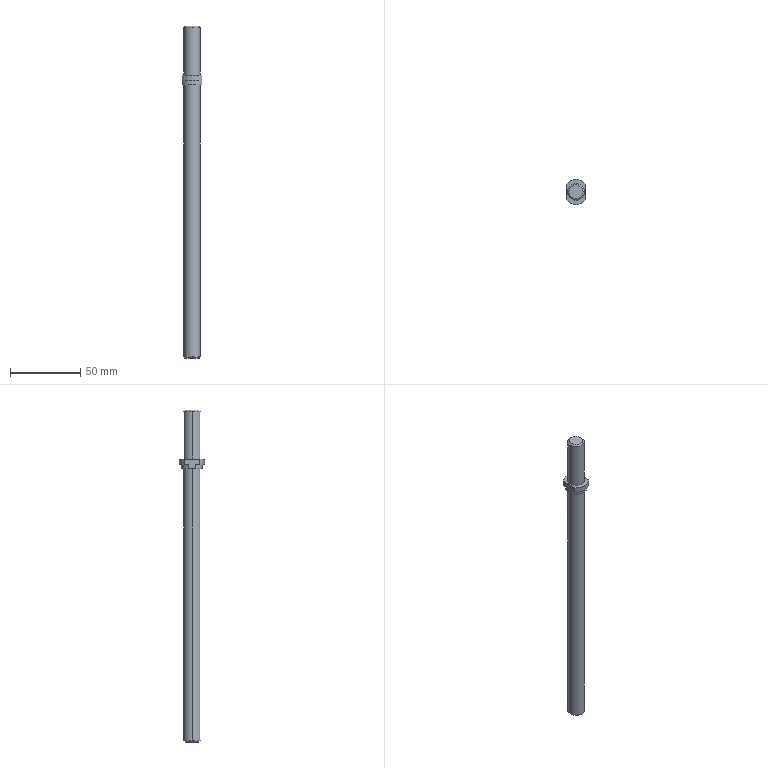Part | STEP file | MT-COMBO-119-S043 | 1 solid | 24 faces | box 14 x 18 x 237 mm | volume 27010 mm3 | cylinder 10 | plane 8 | cone 6 | commonest cylinder face diameters 12 x4 4.2 x2 15 x2 18 x2
STEP:
#1=CARTESIAN_POINT('',(2.1,0.,15.));
#2=VERTEX_POINT('',#1);
#3=CARTESIAN_POINT('',(-2.1,0.,15.));
#4=VERTEX_POINT('',#3);
#5=CARTESIAN_POINT('',(0.,0.,15.));
#6=DIRECTION('',(0.,0.,1.));
#7=DIRECTION('',(1.,0.,0.));
#8=AXIS2_PLACEMENT_3D('',#5,#6,#7);
#9=CIRCLE('',#8,2.1);
#10=EDGE_CURVE('',#2,#4,#9,.T.);
#11=ORIENTED_EDGE('',*,*,#10,.T.);
#12=CARTESIAN_POINT('',(-2.1,0.,-12.));
#13=VERTEX_POINT('',#12);
#14=CARTESIAN_POINT('',(-2.1,0.,0.));
#15=DIRECTION('',(0.,0.,-1.));
#16=VECTOR('',#15,1000.);
#17=LINE('',#14,#16);
#18=EDGE_CURVE('',#4,#13,#17,.T.);
#19=ORIENTED_EDGE('',*,*,#18,.T.);
#20=CARTESIAN_POINT('',(2.1,0.,-12.));
#21=VERTEX_POINT('',#20);
#22=CARTESIAN_POINT('',(0.,0.,-12.));
#23=DIRECTION('',(0.,0.,1.));
#24=DIRECTION('',(1.,0.,0.));
#25=AXIS2_PLACEMENT_3D('',#22,#23,#24);
#26=CIRCLE('',#25,2.1);
#27=EDGE_CURVE('',#21,#13,#26,.T.);
#28=ORIENTED_EDGE('',*,*,#27,.F.);
#29=CARTESIAN_POINT('',(2.1,0.,0.));
#30=DIRECTION('',(0.,0.,-1.));
#31=VECTOR('',#30,1000.);
#32=LINE('',#29,#31);
#33=EDGE_CURVE('',#2,#21,#32,.T.);
#34=ORIENTED_EDGE('',*,*,#33,.F.);
#35=EDGE_LOOP('',(#11,#19,#28,#34));
#36=FACE_OUTER_BOUND('',#35,.T.);
#37=CARTESIAN_POINT('',(0.,0.,0.));
#38=DIRECTION('',(0.,0.,-1.));
#39=DIRECTION('',(1.,0.,0.));
#40=AXIS2_PLACEMENT_3D('',#37,#38,#39);
#41=CYLINDRICAL_SURFACE('',#40,2.1);
#42=ADVANCED_FACE('',(#36),#41,.F.);
#43=CARTESIAN_POINT('',(0.,0.,16.262));
#44=VERTEX_POINT('',#43);
#45=CARTESIAN_POINT('',(2.1,0.,15.));
#46=DIRECTION('',(0.8572,0.,-0.515));
#47=VECTOR('',#46,1000.);
#48=LINE('',#45,#47);
#49=EDGE_CURVE('',#44,#2,#48,.T.);
#50=ORIENTED_EDGE('',*,*,#49,.F.);
#51=CARTESIAN_POINT('',(-2.1,0.,15.));
#52=DIRECTION('',(-0.8572,0.,-0.515));
#53=VECTOR('',#52,1000.);
#54=LINE('',#51,#53);
#55=EDGE_CURVE('',#44,#4,#54,.T.);
#56=ORIENTED_EDGE('',*,*,#55,.T.);
#57=ORIENTED_EDGE('',*,*,#10,.F.);
#58=EDGE_LOOP('',(#50,#56,#57));
#59=FACE_OUTER_BOUND('',#58,.T.);
#60=CARTESIAN_POINT('',(0.,0.,15.));
#61=DIRECTION('',(0.,0.,-1.));
#62=DIRECTION('',(1.,0.,0.));
#63=AXIS2_PLACEMENT_3D('',#60,#61,#62);
#64=CONICAL_SURFACE('',#63,2.1,1.03);
#65=ADVANCED_FACE('',(#59),#64,.F.);
#66=CARTESIAN_POINT('',(-5.,0.,-12.));
#67=VERTEX_POINT('',#66);
#68=CARTESIAN_POINT('',(5.,0.,-12.));
#69=VERTEX_POINT('',#68);
#70=CARTESIAN_POINT('',(0.,0.,-12.));
#71=DIRECTION('',(0.,0.,1.));
#72=DIRECTION('',(1.,0.,0.));
#73=AXIS2_PLACEMENT_3D('',#70,#71,#72);
#74=CIRCLE('',#73,5.);
#75=EDGE_CURVE('',#67,#69,#74,.T.);
#76=ORIENTED_EDGE('',*,*,#75,.T.);
#77=CARTESIAN_POINT('',(6.,0.,-11.));
#78=VERTEX_POINT('',#77);
#79=CARTESIAN_POINT('',(5.,0.,-12.));
#80=DIRECTION('',(0.7071,0.,0.7071));
#81=VECTOR('',#80,1000.);
#82=LINE('',#79,#81);
#83=EDGE_CURVE('',#69,#78,#82,.T.);
#84=ORIENTED_EDGE('',*,*,#83,.T.);
#85=CARTESIAN_POINT('',(-6.,0.,-11.));
#86=VERTEX_POINT('',#85);
#87=CARTESIAN_POINT('',(0.,0.,-11.));
#88=DIRECTION('',(0.,0.,-1.));
#89=DIRECTION('',(1.,0.,0.));
#90=AXIS2_PLACEMENT_3D('',#87,#88,#89);
#91=CIRCLE('',#90,6.);
#92=EDGE_CURVE('',#78,#86,#91,.T.);
#93=ORIENTED_EDGE('',*,*,#92,.T.);
#94=CARTESIAN_POINT('',(-5.,0.,-12.));
#95=DIRECTION('',(-0.7071,0.,0.7071));
#96=VECTOR('',#95,1000.);
#97=LINE('',#94,#96);
#98=EDGE_CURVE('',#67,#86,#97,.T.);
#99=ORIENTED_EDGE('',*,*,#98,.F.);
#100=EDGE_LOOP('',(#76,#84,#93,#99));
#101=FACE_OUTER_BOUND('',#100,.T.);
#102=CARTESIAN_POINT('',(0.,0.,-12.));
#103=DIRECTION('',(0.,0.,1.));
#104=DIRECTION('',(-1.,0.,0.));
#105=AXIS2_PLACEMENT_3D('',#102,#103,#104);
#106=CONICAL_SURFACE('',#105,5.,0.7854);
#107=ADVANCED_FACE('',(#101),#106,.T.);
#108=CARTESIAN_POINT('',(5.,0.,225.));
#109=VERTEX_POINT('',#108);
#110=CARTESIAN_POINT('',(-5.,0.,225.));
#111=VERTEX_POINT('',#110);
#112=CARTESIAN_POINT('',(0.,0.,225.));
#113=DIRECTION('',(0.,0.,-1.));
#114=DIRECTION('',(1.,0.,0.));
#115=AXIS2_PLACEMENT_3D('',#112,#113,#114);
#116=CIRCLE('',#115,5.);
#117=EDGE_CURVE('',#109,#111,#116,.T.);
#118=ORIENTED_EDGE('',*,*,#117,.T.);
#119=CARTESIAN_POINT('',(-6.,0.,224.));
#120=VERTEX_POINT('',#119);
#121=CARTESIAN_POINT('',(-6.,0.,224.));
#122=DIRECTION('',(-0.7071,0.,-0.7071));
#123=VECTOR('',#122,1000.);
#124=LINE('',#121,#123);
#125=EDGE_CURVE('',#111,#120,#124,.T.);
#126=ORIENTED_EDGE('',*,*,#125,.T.);
#127=CARTESIAN_POINT('',(6.,0.,224.));
#128=VERTEX_POINT('',#127);
#129=CARTESIAN_POINT('',(0.,0.,224.));
#130=DIRECTION('',(0.,0.,1.));
#131=DIRECTION('',(1.,0.,0.));
#132=AXIS2_PLACEMENT_3D('',#129,#130,#131);
#133=CIRCLE('',#132,6.);
#134=EDGE_CURVE('',#120,#128,#133,.T.);
#135=ORIENTED_EDGE('',*,*,#134,.T.);
#136=CARTESIAN_POINT('',(6.,0.,224.));
#137=DIRECTION('',(0.7071,0.,-0.7071));
#138=VECTOR('',#137,1000.);
#139=LINE('',#136,#138);
#140=EDGE_CURVE('',#109,#128,#139,.T.);
#141=ORIENTED_EDGE('',*,*,#140,.F.);
#142=EDGE_LOOP('',(#118,#126,#135,#141));
#143=FACE_OUTER_BOUND('',#142,.T.);
#144=CARTESIAN_POINT('',(0.,0.,224.));
#145=DIRECTION('',(0.,0.,-1.));
#146=DIRECTION('',(1.,0.,0.));
#147=AXIS2_PLACEMENT_3D('',#144,#145,#146);
#148=CONICAL_SURFACE('',#147,6.,0.7854);
#149=ADVANCED_FACE('',(#143),#148,.T.);
#150=CARTESIAN_POINT('',(-6.,0.,183.));
#151=VERTEX_POINT('',#150);
#152=CARTESIAN_POINT('',(6.,0.,183.));
#153=VERTEX_POINT('',#152);
#154=CARTESIAN_POINT('',(0.,0.,183.));
#155=DIRECTION('',(0.,0.,1.));
#156=DIRECTION('',(-1.,0.,0.));
#157=AXIS2_PLACEMENT_3D('',#154,#155,#156);
#158=CIRCLE('',#157,6.);
#159=EDGE_CURVE('',#151,#153,#158,.T.);
#160=ORIENTED_EDGE('',*,*,#159,.F.);
#161=CARTESIAN_POINT('',(-6.,0.,225.));
#162=DIRECTION('',(0.,0.,-1.));
#163=VECTOR('',#162,1000.);
#164=LINE('',#161,#163);
#165=EDGE_CURVE('',#151,#86,#164,.T.);
#166=ORIENTED_EDGE('',*,*,#165,.T.);
#167=ORIENTED_EDGE('',*,*,#92,.F.);
#168=CARTESIAN_POINT('',(6.,0.,225.));
#169=DIRECTION('',(0.,0.,-1.));
#170=VECTOR('',#169,1000.);
#171=LINE('',#168,#170);
#172=EDGE_CURVE('',#153,#78,#171,.T.);
#173=ORIENTED_EDGE('',*,*,#172,.F.);
#174=EDGE_LOOP('',(#160,#166,#167,#173));
#175=FACE_OUTER_BOUND('',#174,.T.);
#176=CARTESIAN_POINT('',(0.,0.,225.));
#177=DIRECTION('',(0.,0.,-1.));
#178=DIRECTION('',(1.,0.,0.));
#179=AXIS2_PLACEMENT_3D('',#176,#177,#178);
#180=CYLINDRICAL_SURFACE('',#179,6.);
#181=ADVANCED_FACE('',(#175),#180,.T.);
#182=ORIENTED_EDGE('',*,*,#134,.F.);
#183=CARTESIAN_POINT('',(-6.,0.,190.));
#184=VERTEX_POINT('',#183);
#185=CARTESIAN_POINT('',(-6.,0.,225.));
#186=DIRECTION('',(0.,0.,-1.));
#187=VECTOR('',#186,1000.);
#188=LINE('',#185,#187);
#189=EDGE_CURVE('',#120,#184,#188,.T.);
#190=ORIENTED_EDGE('',*,*,#189,.T.);
#191=CARTESIAN_POINT('',(6.,0.,190.));
#192=VERTEX_POINT('',#191);
#193=CARTESIAN_POINT('',(0.,0.,190.));
#194=DIRECTION('',(0.,0.,-1.));
#195=DIRECTION('',(1.,0.,0.));
#196=AXIS2_PLACEMENT_3D('',#193,#194,#195);
#197=CIRCLE('',#196,6.);
#198=EDGE_CURVE('',#192,#184,#197,.T.);
#199=ORIENTED_EDGE('',*,*,#198,.F.);
#200=CARTESIAN_POINT('',(6.,0.,225.));
#201=DIRECTION('',(0.,0.,-1.));
#202=VECTOR('',#201,1000.);
#203=LINE('',#200,#202);
#204=EDGE_CURVE('',#128,#192,#203,.T.);
#205=ORIENTED_EDGE('',*,*,#204,.F.);
#206=EDGE_LOOP('',(#182,#190,#199,#205));
#207=FACE_OUTER_BOUND('',#206,.T.);
#208=CARTESIAN_POINT('',(0.,0.,225.));
#209=DIRECTION('',(0.,0.,-1.));
#210=DIRECTION('',(1.,0.,0.));
#211=AXIS2_PLACEMENT_3D('',#208,#209,#210);
#212=CYLINDRICAL_SURFACE('',#211,6.);
#213=ADVANCED_FACE('',(#207),#212,.T.);
#214=CARTESIAN_POINT('',(-7.,5.657,186.));
#215=VERTEX_POINT('',#214);
#216=CARTESIAN_POINT('',(7.,5.657,186.));
#217=VERTEX_POINT('',#216);
#218=CARTESIAN_POINT('',(0.,0.,186.));
#219=DIRECTION('',(0.,0.,-1.));
#220=DIRECTION('',(-1.,0.,0.));
#221=AXIS2_PLACEMENT_3D('',#218,#219,#220);
#222=CIRCLE('',#221,9.);
#223=EDGE_CURVE('',#215,#217,#222,.T.);
#224=ORIENTED_EDGE('',*,*,#223,.F.);
#225=CARTESIAN_POINT('',(-7.,5.657,190.));
#226=VERTEX_POINT('',#225);
#227=CARTESIAN_POINT('',(-7.,5.657,225.));
#228=DIRECTION('',(0.,0.,-1.));
#229=VECTOR('',#228,1000.);
#230=LINE('',#227,#229);
#231=EDGE_CURVE('',#226,#215,#230,.T.);
#232=ORIENTED_EDGE('',*,*,#231,.F.);
#233=CARTESIAN_POINT('',(7.,5.657,190.));
#234=VERTEX_POINT('',#233);
#235=CARTESIAN_POINT('',(0.,0.,190.));
#236=DIRECTION('',(0.,0.,-1.));
#237=DIRECTION('',(-1.,0.,0.));
#238=AXIS2_PLACEMENT_3D('',#235,#236,#237);
#239=CIRCLE('',#238,9.);
#240=EDGE_CURVE('',#226,#234,#239,.T.);
#241=ORIENTED_EDGE('',*,*,#240,.T.);
#242=CARTESIAN_POINT('',(7.,5.657,225.));
#243=DIRECTION('',(0.,0.,1.));
#244=VECTOR('',#243,1000.);
#245=LINE('',#242,#244);
#246=EDGE_CURVE('',#217,#234,#245,.T.);
#247=ORIENTED_EDGE('',*,*,#246,.F.);
#248=EDGE_LOOP('',(#224,#232,#241,#247));
#249=FACE_OUTER_BOUND('',#248,.T.);
#250=CARTESIAN_POINT('',(0.,0.,225.));
#251=DIRECTION('',(0.,0.,1.));
#252=DIRECTION('',(-1.,0.,0.));
#253=AXIS2_PLACEMENT_3D('',#250,#251,#252);
#254=CYLINDRICAL_SURFACE('',#253,9.);
#255=ADVANCED_FACE('',(#249),#254,.T.);
#256=CARTESIAN_POINT('',(7.,-5.657,186.));
#257=VERTEX_POINT('',#256);
#258=CARTESIAN_POINT('',(-7.,-5.657,186.));
#259=VERTEX_POINT('',#258);
#260=CARTESIAN_POINT('',(0.,0.,186.));
#261=DIRECTION('',(0.,0.,-1.));
#262=DIRECTION('',(-1.,0.,0.));
#263=AXIS2_PLACEMENT_3D('',#260,#261,#262);
#264=CIRCLE('',#263,9.);
#265=EDGE_CURVE('',#257,#259,#264,.T.);
#266=ORIENTED_EDGE('',*,*,#265,.T.);
#267=CARTESIAN_POINT('',(-7.,-2.693,186.));
#268=VERTEX_POINT('',#267);
#269=CARTESIAN_POINT('',(-7.,0.,186.));
#270=DIRECTION('',(0.,-1.,0.));
#271=VECTOR('',#270,1000.);
#272=LINE('',#269,#271);
#273=EDGE_CURVE('',#268,#259,#272,.T.);
#274=ORIENTED_EDGE('',*,*,#273,.F.);
#275=CARTESIAN_POINT('',(7.,-2.693,186.));
#276=VERTEX_POINT('',#275);
#277=CARTESIAN_POINT('',(0.,0.,186.));
#278=DIRECTION('',(0.,0.,-1.));
#279=DIRECTION('',(-1.,0.,0.));
#280=AXIS2_PLACEMENT_3D('',#277,#278,#279);
#281=CIRCLE('',#280,7.5);
#282=EDGE_CURVE('',#276,#268,#281,.T.);
#283=ORIENTED_EDGE('',*,*,#282,.F.);
#284=CARTESIAN_POINT('',(7.,0.,186.));
#285=DIRECTION('',(0.,1.,0.));
#286=VECTOR('',#285,1000.);
#287=LINE('',#284,#286);
#288=EDGE_CURVE('',#257,#276,#287,.T.);
#289=ORIENTED_EDGE('',*,*,#288,.F.);
#290=EDGE_LOOP('',(#266,#274,#283,#289));
#291=FACE_OUTER_BOUND('',#290,.T.);
#292=CARTESIAN_POINT('',(7.5,0.,186.));
#293=DIRECTION('',(0.,0.,1.));
#294=DIRECTION('',(-1.,0.,0.));
#295=AXIS2_PLACEMENT_3D('',#292,#293,#294);
#296=PLANE('',#295);
#297=ADVANCED_FACE('',(#291),#296,.F.);
#298=CARTESIAN_POINT('',(-7.,2.693,183.));
#299=VERTEX_POINT('',#298);
#300=CARTESIAN_POINT('',(7.,2.693,183.));
#301=VERTEX_POINT('',#300);
#302=CARTESIAN_POINT('',(0.,0.,183.));
#303=DIRECTION('',(0.,0.,-1.));
#304=DIRECTION('',(-1.,0.,0.));
#305=AXIS2_PLACEMENT_3D('',#302,#303,#304);
#306=CIRCLE('',#305,7.5);
#307=EDGE_CURVE('',#299,#301,#306,.T.);
#308=ORIENTED_EDGE('',*,*,#307,.F.);
#309=CARTESIAN_POINT('',(-7.,2.693,186.));
#310=VERTEX_POINT('',#309);
#311=CARTESIAN_POINT('',(-7.,2.693,225.));
#312=DIRECTION('',(0.,0.,-1.));
#313=VECTOR('',#312,1000.);
#314=LINE('',#311,#313);
#315=EDGE_CURVE('',#310,#299,#314,.T.);
#316=ORIENTED_EDGE('',*,*,#315,.F.);
#317=CARTESIAN_POINT('',(7.,2.693,186.));
#318=VERTEX_POINT('',#317);
#319=CARTESIAN_POINT('',(0.,0.,186.));
#320=DIRECTION('',(0.,0.,-1.));
#321=DIRECTION('',(-1.,0.,0.));
#322=AXIS2_PLACEMENT_3D('',#319,#320,#321);
#323=CIRCLE('',#322,7.5);
#324=EDGE_CURVE('',#310,#318,#323,.T.);
#325=ORIENTED_EDGE('',*,*,#324,.T.);
#326=CARTESIAN_POINT('',(7.,2.693,225.));
#327=DIRECTION('',(0.,0.,1.));
#328=VECTOR('',#327,1000.);
#329=LINE('',#326,#328);
#330=EDGE_CURVE('',#301,#318,#329,.T.);
#331=ORIENTED_EDGE('',*,*,#330,.F.);
#332=EDGE_LOOP('',(#308,#316,#325,#331));
#333=FACE_OUTER_BOUND('',#332,.T.);
#334=CARTESIAN_POINT('',(0.,0.,225.));
#335=DIRECTION('',(0.,0.,1.));
#336=DIRECTION('',(-1.,0.,0.));
#337=AXIS2_PLACEMENT_3D('',#334,#335,#336);
#338=CYLINDRICAL_SURFACE('',#337,7.5);
#339=ADVANCED_FACE('',(#333),#338,.T.);
#340=ORIENTED_EDGE('',*,*,#189,.F.);
#341=CARTESIAN_POINT('',(0.,0.,224.));
#342=DIRECTION('',(0.,0.,1.));
#343=DIRECTION('',(1.,0.,0.));
#344=AXIS2_PLACEMENT_3D('',#341,#342,#343);
#345=CIRCLE('',#344,6.);
#346=EDGE_CURVE('',#128,#120,#345,.T.);
#347=ORIENTED_EDGE('',*,*,#346,.F.);
#348=ORIENTED_EDGE('',*,*,#204,.T.);
#349=CARTESIAN_POINT('',(0.,0.,190.));
#350=DIRECTION('',(0.,0.,-1.));
#351=DIRECTION('',(1.,0.,0.));
#352=AXIS2_PLACEMENT_3D('',#349,#350,#351);
#353=CIRCLE('',#352,6.);
#354=EDGE_CURVE('',#184,#192,#353,.T.);
#355=ORIENTED_EDGE('',*,*,#354,.F.);
#356=EDGE_LOOP('',(#340,#347,#348,#355));
#357=FACE_OUTER_BOUND('',#356,.T.);
#358=CARTESIAN_POINT('',(0.,0.,225.));
#359=DIRECTION('',(0.,0.,-1.));
#360=DIRECTION('',(1.,0.,0.));
#361=AXIS2_PLACEMENT_3D('',#358,#359,#360);
#362=CYLINDRICAL_SURFACE('',#361,6.);
#363=ADVANCED_FACE('',(#357),#362,.T.);
#364=ORIENTED_EDGE('',*,*,#117,.F.);
#365=CARTESIAN_POINT('',(0.,0.,225.));
#366=DIRECTION('',(0.,0.,-1.));
#367=DIRECTION('',(1.,0.,0.));
#368=AXIS2_PLACEMENT_3D('',#365,#366,#367);
#369=CIRCLE('',#368,5.);
#370=EDGE_CURVE('',#111,#109,#369,.T.);
#371=ORIENTED_EDGE('',*,*,#370,.F.);
#372=EDGE_LOOP('',(#364,#371));
#373=FACE_OUTER_BOUND('',#372,.T.);
#374=CARTESIAN_POINT('',(0.,0.,225.));
#375=DIRECTION('',(0.,0.,-1.));
#376=DIRECTION('',(1.,0.,0.));
#377=AXIS2_PLACEMENT_3D('',#374,#375,#376);
#378=PLANE('',#377);
#379=ADVANCED_FACE('',(#373),#378,.F.);
#380=ORIENTED_EDGE('',*,*,#198,.T.);
#381=ORIENTED_EDGE('',*,*,#354,.T.);
#382=EDGE_LOOP('',(#380,#381));
#383=FACE_BOUND('',#382,.T.);
#384=ORIENTED_EDGE('',*,*,#240,.F.);
#385=CARTESIAN_POINT('',(-7.,-5.657,190.));
#386=VERTEX_POINT('',#385);
#387=CARTESIAN_POINT('',(-7.,14.131,190.));
#388=DIRECTION('',(0.,-1.,0.));
#389=VECTOR('',#388,1000.);
#390=LINE('',#387,#389);
#391=EDGE_CURVE('',#226,#386,#390,.T.);
#392=ORIENTED_EDGE('',*,*,#391,.T.);
#393=CARTESIAN_POINT('',(7.,-5.657,190.));
#394=VERTEX_POINT('',#393);
#395=CARTESIAN_POINT('',(0.,0.,190.));
#396=DIRECTION('',(0.,0.,-1.));
#397=DIRECTION('',(-1.,0.,0.));
#398=AXIS2_PLACEMENT_3D('',#395,#396,#397);
#399=CIRCLE('',#398,9.);
#400=EDGE_CURVE('',#394,#386,#399,.T.);
#401=ORIENTED_EDGE('',*,*,#400,.F.);
#402=CARTESIAN_POINT('',(7.,14.131,190.));
#403=DIRECTION('',(0.,1.,0.));
#404=VECTOR('',#403,1000.);
#405=LINE('',#402,#404);
#406=EDGE_CURVE('',#394,#234,#405,.T.);
#407=ORIENTED_EDGE('',*,*,#406,.T.);
#408=EDGE_LOOP('',(#384,#392,#401,#407));
#409=FACE_OUTER_BOUND('',#408,.T.);
#410=CARTESIAN_POINT('',(0.,0.,190.));
#411=DIRECTION('',(0.,0.,-1.));
#412=DIRECTION('',(1.,0.,0.));
#413=AXIS2_PLACEMENT_3D('',#410,#411,#412);
#414=PLANE('',#413);
#415=ADVANCED_FACE('',(#383,#409),#414,.F.);
#416=ORIENTED_EDGE('',*,*,#400,.T.);
#417=CARTESIAN_POINT('',(-7.,-5.657,225.));
#418=DIRECTION('',(0.,0.,1.));
#419=VECTOR('',#418,1000.);
#420=LINE('',#417,#419);
#421=EDGE_CURVE('',#259,#386,#420,.T.);
#422=ORIENTED_EDGE('',*,*,#421,.F.);
#423=ORIENTED_EDGE('',*,*,#265,.F.);
#424=CARTESIAN_POINT('',(7.,-5.657,225.));
#425=DIRECTION('',(0.,0.,-1.));
#426=VECTOR('',#425,1000.);
#427=LINE('',#424,#426);
#428=EDGE_CURVE('',#394,#257,#427,.T.);
#429=ORIENTED_EDGE('',*,*,#428,.F.);
#430=EDGE_LOOP('',(#416,#422,#423,#429));
#431=FACE_OUTER_BOUND('',#430,.T.);
#432=CARTESIAN_POINT('',(0.,0.,225.));
#433=DIRECTION('',(0.,0.,1.));
#434=DIRECTION('',(-1.,0.,0.));
#435=AXIS2_PLACEMENT_3D('',#432,#433,#434);
#436=CYLINDRICAL_SURFACE('',#435,9.);
#437=ADVANCED_FACE('',(#431),#436,.T.);
#438=ORIENTED_EDGE('',*,*,#324,.F.);
#439=CARTESIAN_POINT('',(-7.,0.,186.));
#440=DIRECTION('',(0.,-1.,0.));
#441=VECTOR('',#440,1000.);
#442=LINE('',#439,#441);
#443=EDGE_CURVE('',#215,#310,#442,.T.);
#444=ORIENTED_EDGE('',*,*,#443,.F.);
#445=ORIENTED_EDGE('',*,*,#223,.T.);
#446=CARTESIAN_POINT('',(7.,0.,186.));
#447=DIRECTION('',(0.,1.,0.));
#448=VECTOR('',#447,1000.);
#449=LINE('',#446,#448);
#450=EDGE_CURVE('',#318,#217,#449,.T.);
#451=ORIENTED_EDGE('',*,*,#450,.F.);
#452=EDGE_LOOP('',(#438,#444,#445,#451));
#453=FACE_OUTER_BOUND('',#452,.T.);
#454=CARTESIAN_POINT('',(7.5,0.,186.));
#455=DIRECTION('',(0.,0.,1.));
#456=DIRECTION('',(-1.,0.,0.));
#457=AXIS2_PLACEMENT_3D('',#454,#455,#456);
#458=PLANE('',#457);
#459=ADVANCED_FACE('',(#453),#458,.F.);
#460=ORIENTED_EDGE('',*,*,#282,.T.);
#461=CARTESIAN_POINT('',(-7.,-2.693,183.));
#462=VERTEX_POINT('',#461);
#463=CARTESIAN_POINT('',(-7.,-2.693,225.));
#464=DIRECTION('',(0.,0.,1.));
#465=VECTOR('',#464,1000.);
#466=LINE('',#463,#465);
#467=EDGE_CURVE('',#462,#268,#466,.T.);
#468=ORIENTED_EDGE('',*,*,#467,.F.);
#469=CARTESIAN_POINT('',(7.,-2.693,183.));
#470=VERTEX_POINT('',#469);
#471=CARTESIAN_POINT('',(0.,0.,183.));
#472=DIRECTION('',(0.,0.,-1.));
#473=DIRECTION('',(-1.,0.,0.));
#474=AXIS2_PLACEMENT_3D('',#471,#472,#473);
#475=CIRCLE('',#474,7.5);
#476=EDGE_CURVE('',#470,#462,#475,.T.);
#477=ORIENTED_EDGE('',*,*,#476,.F.);
#478=CARTESIAN_POINT('',(7.,-2.693,225.));
#479=DIRECTION('',(0.,0.,-1.));
#480=VECTOR('',#479,1000.);
#481=LINE('',#478,#480);
#482=EDGE_CURVE('',#276,#470,#481,.T.);
#483=ORIENTED_EDGE('',*,*,#482,.F.);
#484=EDGE_LOOP('',(#460,#468,#477,#483));
#485=FACE_OUTER_BOUND('',#484,.T.);
#486=CARTESIAN_POINT('',(0.,0.,225.));
#487=DIRECTION('',(0.,0.,1.));
#488=DIRECTION('',(-1.,0.,0.));
#489=AXIS2_PLACEMENT_3D('',#486,#487,#488);
#490=CYLINDRICAL_SURFACE('',#489,7.5);
#491=ADVANCED_FACE('',(#485),#490,.T.);
#492=CARTESIAN_POINT('',(0.,0.,183.));
#493=DIRECTION('',(0.,0.,1.));
#494=DIRECTION('',(-1.,0.,0.));
#495=AXIS2_PLACEMENT_3D('',#492,#493,#494);
#496=CIRCLE('',#495,6.);
#497=EDGE_CURVE('',#153,#151,#496,.T.);
#498=ORIENTED_EDGE('',*,*,#497,.T.);
#499=ORIENTED_EDGE('',*,*,#159,.T.);
#500=EDGE_LOOP('',(#498,#499));
#501=FACE_BOUND('',#500,.T.);
#502=ORIENTED_EDGE('',*,*,#476,.T.);
#503=CARTESIAN_POINT('',(-7.,0.,183.));
#504=DIRECTION('',(0.,-1.,0.));
#505=VECTOR('',#504,1000.);
#506=LINE('',#503,#505);
#507=EDGE_CURVE('',#299,#462,#506,.T.);
#508=ORIENTED_EDGE('',*,*,#507,.F.);
#509=ORIENTED_EDGE('',*,*,#307,.T.);
#510=CARTESIAN_POINT('',(7.,0.,183.));
#511=DIRECTION('',(0.,1.,0.));
#512=VECTOR('',#511,1000.);
#513=LINE('',#510,#512);
#514=EDGE_CURVE('',#470,#301,#513,.T.);
#515=ORIENTED_EDGE('',*,*,#514,.F.);
#516=EDGE_LOOP('',(#502,#508,#509,#515));
#517=FACE_OUTER_BOUND('',#516,.T.);
#518=CARTESIAN_POINT('',(7.5,0.,183.));
#519=DIRECTION('',(0.,0.,1.));
#520=DIRECTION('',(-1.,0.,0.));
#521=AXIS2_PLACEMENT_3D('',#518,#519,#520);
#522=PLANE('',#521);
#523=ADVANCED_FACE('',(#501,#517),#522,.F.);
#524=ORIENTED_EDGE('',*,*,#27,.T.);
#525=CARTESIAN_POINT('',(0.,0.,-12.));
#526=DIRECTION('',(0.,0.,1.));
#527=DIRECTION('',(1.,0.,0.));
#528=AXIS2_PLACEMENT_3D('',#525,#526,#527);
#529=CIRCLE('',#528,2.1);
#530=EDGE_CURVE('',#13,#21,#529,.T.);
#531=ORIENTED_EDGE('',*,*,#530,.T.);
#532=EDGE_LOOP('',(#524,#531));
#533=FACE_BOUND('',#532,.T.);
#534=ORIENTED_EDGE('',*,*,#75,.F.);
#535=CARTESIAN_POINT('',(0.,0.,-12.));
#536=DIRECTION('',(0.,0.,1.));
#537=DIRECTION('',(1.,0.,0.));
#538=AXIS2_PLACEMENT_3D('',#535,#536,#537);
#539=CIRCLE('',#538,5.);
#540=EDGE_CURVE('',#69,#67,#539,.T.);
#541=ORIENTED_EDGE('',*,*,#540,.F.);
#542=EDGE_LOOP('',(#534,#541));
#543=FACE_OUTER_BOUND('',#542,.T.);
#544=CARTESIAN_POINT('',(0.,0.,-12.));
#545=DIRECTION('',(0.,0.,-1.));
#546=DIRECTION('',(1.,0.,0.));
#547=AXIS2_PLACEMENT_3D('',#544,#545,#546);
#548=PLANE('',#547);
#549=ADVANCED_FACE('',(#533,#543),#548,.T.);
#550=ORIENTED_EDGE('',*,*,#165,.F.);
#551=ORIENTED_EDGE('',*,*,#497,.F.);
#552=ORIENTED_EDGE('',*,*,#172,.T.);
#553=CARTESIAN_POINT('',(0.,0.,-11.));
#554=DIRECTION('',(0.,0.,-1.));
#555=DIRECTION('',(1.,0.,0.));
#556=AXIS2_PLACEMENT_3D('',#553,#554,#555);
#557=CIRCLE('',#556,6.);
#558=EDGE_CURVE('',#86,#78,#557,.T.);
#559=ORIENTED_EDGE('',*,*,#558,.F.);
#560=EDGE_LOOP('',(#550,#551,#552,#559));
#561=FACE_OUTER_BOUND('',#560,.T.);
#562=CARTESIAN_POINT('',(0.,0.,225.));
#563=DIRECTION('',(0.,0.,-1.));
#564=DIRECTION('',(1.,0.,0.));
#565=AXIS2_PLACEMENT_3D('',#562,#563,#564);
#566=CYLINDRICAL_SURFACE('',#565,6.);
#567=ADVANCED_FACE('',(#561),#566,.T.);
#568=ORIENTED_EDGE('',*,*,#125,.F.);
#569=ORIENTED_EDGE('',*,*,#370,.T.);
#570=ORIENTED_EDGE('',*,*,#140,.T.);
#571=ORIENTED_EDGE('',*,*,#346,.T.);
#572=EDGE_LOOP('',(#568,#569,#570,#571));
#573=FACE_OUTER_BOUND('',#572,.T.);
#574=CARTESIAN_POINT('',(0.,0.,224.));
#575=DIRECTION('',(0.,0.,-1.));
#576=DIRECTION('',(1.,0.,0.));
#577=AXIS2_PLACEMENT_3D('',#574,#575,#576);
#578=CONICAL_SURFACE('',#577,6.,0.7854);
#579=ADVANCED_FACE('',(#573),#578,.T.);
#580=ORIENTED_EDGE('',*,*,#83,.F.);
#581=ORIENTED_EDGE('',*,*,#540,.T.);
#582=ORIENTED_EDGE('',*,*,#98,.T.);
#583=ORIENTED_EDGE('',*,*,#558,.T.);
#584=EDGE_LOOP('',(#580,#581,#582,#583));
#585=FACE_OUTER_BOUND('',#584,.T.);
#586=CARTESIAN_POINT('',(0.,0.,-12.));
#587=DIRECTION('',(0.,0.,1.));
#588=DIRECTION('',(-1.,0.,0.));
#589=AXIS2_PLACEMENT_3D('',#586,#587,#588);
#590=CONICAL_SURFACE('',#589,5.,0.7854);
#591=ADVANCED_FACE('',(#585),#590,.T.);
#592=ORIENTED_EDGE('',*,*,#55,.F.);
#593=ORIENTED_EDGE('',*,*,#49,.T.);
#594=CARTESIAN_POINT('',(0.,0.,15.));
#595=DIRECTION('',(0.,0.,1.));
#596=DIRECTION('',(1.,0.,0.));
#597=AXIS2_PLACEMENT_3D('',#594,#595,#596);
#598=CIRCLE('',#597,2.1);
#599=EDGE_CURVE('',#4,#2,#598,.T.);
#600=ORIENTED_EDGE('',*,*,#599,.F.);
#601=EDGE_LOOP('',(#592,#593,#600));
#602=FACE_OUTER_BOUND('',#601,.T.);
#603=CARTESIAN_POINT('',(0.,0.,15.));
#604=DIRECTION('',(0.,0.,-1.));
#605=DIRECTION('',(1.,0.,0.));
#606=AXIS2_PLACEMENT_3D('',#603,#604,#605);
#607=CONICAL_SURFACE('',#606,2.1,1.03);
#608=ADVANCED_FACE('',(#602),#607,.F.);
#609=ORIENTED_EDGE('',*,*,#18,.F.);
#610=ORIENTED_EDGE('',*,*,#599,.T.);
#611=ORIENTED_EDGE('',*,*,#33,.T.);
#612=ORIENTED_EDGE('',*,*,#530,.F.);
#613=EDGE_LOOP('',(#609,#610,#611,#612));
#614=FACE_OUTER_BOUND('',#613,.T.);
#615=CARTESIAN_POINT('',(0.,0.,0.));
#616=DIRECTION('',(0.,0.,-1.));
#617=DIRECTION('',(1.,0.,0.));
#618=AXIS2_PLACEMENT_3D('',#615,#616,#617);
#619=CYLINDRICAL_SURFACE('',#618,2.1);
#620=ADVANCED_FACE('',(#614),#619,.F.);
#621=ORIENTED_EDGE('',*,*,#273,.T.);
#622=ORIENTED_EDGE('',*,*,#421,.T.);
#623=ORIENTED_EDGE('',*,*,#391,.F.);
#624=ORIENTED_EDGE('',*,*,#231,.T.);
#625=ORIENTED_EDGE('',*,*,#443,.T.);
#626=ORIENTED_EDGE('',*,*,#315,.T.);
#627=ORIENTED_EDGE('',*,*,#507,.T.);
#628=ORIENTED_EDGE('',*,*,#467,.T.);
#629=EDGE_LOOP('',(#621,#622,#623,#624,#625,#626,#627,#628));
#630=FACE_OUTER_BOUND('',#629,.T.);
#631=CARTESIAN_POINT('',(-7.,14.131,168.));
#632=DIRECTION('',(1.,0.,0.));
#633=DIRECTION('',(0.,0.,1.));
#634=AXIS2_PLACEMENT_3D('',#631,#632,#633);
#635=PLANE('',#634);
#636=ADVANCED_FACE('',(#630),#635,.F.);
#637=ORIENTED_EDGE('',*,*,#450,.T.);
#638=ORIENTED_EDGE('',*,*,#246,.T.);
#639=ORIENTED_EDGE('',*,*,#406,.F.);
#640=ORIENTED_EDGE('',*,*,#428,.T.);
#641=ORIENTED_EDGE('',*,*,#288,.T.);
#642=ORIENTED_EDGE('',*,*,#482,.T.);
#643=ORIENTED_EDGE('',*,*,#514,.T.);
#644=ORIENTED_EDGE('',*,*,#330,.T.);
#645=EDGE_LOOP('',(#637,#638,#639,#640,#641,#642,#643,#644));
#646=FACE_OUTER_BOUND('',#645,.T.);
#647=CARTESIAN_POINT('',(7.,14.131,168.));
#648=DIRECTION('',(-1.,0.,0.));
#649=DIRECTION('',(0.,0.,-1.));
#650=AXIS2_PLACEMENT_3D('',#647,#648,#649);
#651=PLANE('',#650);
#652=ADVANCED_FACE('',(#646),#651,.F.);
#653=CLOSED_SHELL('',(#42,#65,#107,#149,#181,#213,#255,#297,#339,#363,#379,#415,#437,#459,#491,#523,#549,#567,#579,#591,#608,#620,#636,#652));
#654=MANIFOLD_SOLID_BREP('',#653);
#655=CARTESIAN_POINT('',(0.,0.,0.));
#656=DIRECTION('',(0.,0.,1.));
#657=DIRECTION('',(1.,0.,0.));
#658=AXIS2_PLACEMENT_3D('',#655,#656,#657);
#659=(LENGTH_UNIT()NAMED_UNIT(*)SI_UNIT(.MILLI.,.METRE.));
#660=UNCERTAINTY_MEASURE_WITH_UNIT(LENGTH_MEASURE(0.00001),#659,'','');
#661=(NAMED_UNIT(*)PLANE_ANGLE_UNIT()SI_UNIT($,.RADIAN.));
#662=(NAMED_UNIT(*)SI_UNIT($,.STERADIAN.)SOLID_ANGLE_UNIT());
#663=(GEOMETRIC_REPRESENTATION_CONTEXT(3)GLOBAL_UNCERTAINTY_ASSIGNED_CONTEXT((#660))GLOBAL_UNIT_ASSIGNED_CONTEXT((#659,#661,#662))REPRESENTATION_CONTEXT('',''));
#664=ADVANCED_BREP_SHAPE_REPRESENTATION('',(#654,#658),#663);